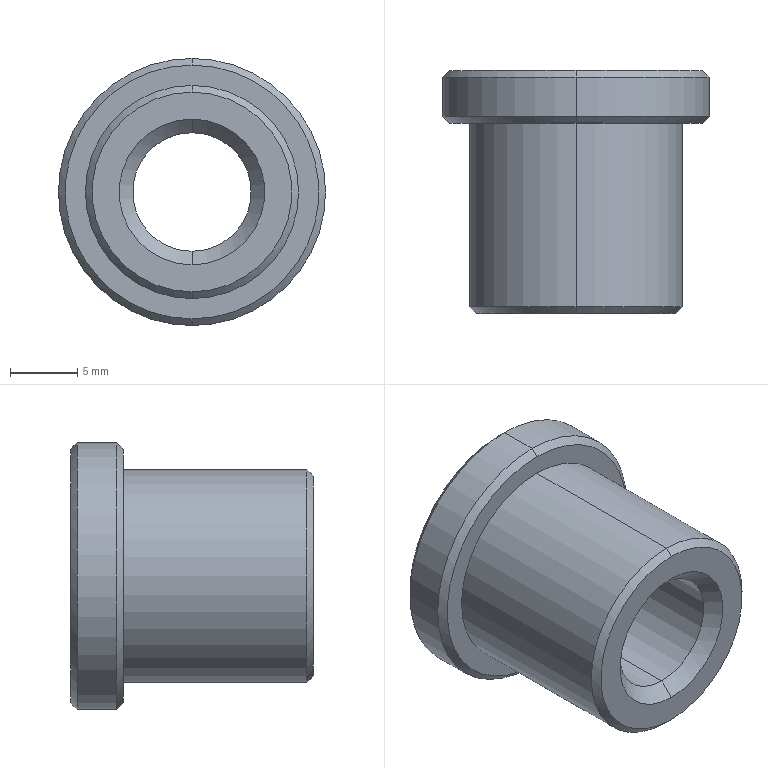Part | STEP file | BPSP-03-039Lift Joint | 1 solid | 19 faces | box 19.8 x 18 x 19.8 mm | volume 2819 mm3 | cone 10 | cylinder 6 | plane 3 | commonest cylinder face diameters 8.8 x2 15.8 x2 19.8 x2
STEP:
#1=CARTESIAN_POINT('',(0.,0.,0.));
#2=DIRECTION('',(0.,0.,1.));
#3=DIRECTION('',(1.,0.,0.));
#4=AXIS2_PLACEMENT_3D('',#1,#2,#3);
#5=CARTESIAN_POINT('',(0.,0.,-7.4));
#6=VERTEX_POINT('',#5);
#7=CARTESIAN_POINT('',(0.,0.,7.4));
#8=VERTEX_POINT('',#7);
#9=CARTESIAN_POINT('',(0.,0.,0.));
#10=DIRECTION('',(0.,-1.,0.));
#11=DIRECTION('',(0.,0.,-1.));
#12=AXIS2_PLACEMENT_3D('',#9,#10,#11);
#13=CIRCLE('',#12,7.4);
#14=CARTESIAN_POINT('',(0.,0.5,0.));
#15=DIRECTION('',(0.,1.,0.));
#16=DIRECTION('',(0.,0.,1.));
#17=AXIS2_PLACEMENT_3D('',#14,#15,#16);
#18=CONICAL_SURFACE('',#17,7.9,0.7854);
#19=CARTESIAN_POINT('',(3.142,-0.5));
#20=DIRECTION('',(-1.,0.));
#21=VECTOR('',#20,1.);
#22=LINE('',#19,#21);
#23=(GEOMETRIC_REPRESENTATION_CONTEXT(2)PARAMETRIC_REPRESENTATION_CONTEXT()REPRESENTATION_CONTEXT('',''));
#24=DEFINITIONAL_REPRESENTATION('',(#22),#23);
#25=PCURVE('',#18,#24);
#26=CARTESIAN_POINT('',(-4.,0.,0.));
#27=DIRECTION('',(0.,-1.,0.));
#28=DIRECTION('',(0.,0.,-1.));
#29=AXIS2_PLACEMENT_3D('',#26,#27,#28);
#30=PLANE('',#29);
#31=CARTESIAN_POINT('',(0.,4.));
#32=DIRECTION('',(1.,0.));
#33=AXIS2_PLACEMENT_2D('',#31,#32);
#34=CIRCLE('',#33,7.4);
#35=(GEOMETRIC_REPRESENTATION_CONTEXT(2)PARAMETRIC_REPRESENTATION_CONTEXT()REPRESENTATION_CONTEXT('',''));
#36=DEFINITIONAL_REPRESENTATION('',(#34),#35);
#37=PCURVE('',#30,#36);
#38=SURFACE_CURVE('',#13,(#25,#37),.PCURVE_S1.);
#39=EDGE_CURVE('',#6,#8,#38,.T.);
#40=ORIENTED_EDGE('',*,*,#39,.F.);
#41=CARTESIAN_POINT('',(0.,0.5,-7.9));
#42=VERTEX_POINT('',#41);
#43=CARTESIAN_POINT('',(0.,0.5,-7.9));
#44=DIRECTION('',(0.,0.7071,-0.7071));
#45=VECTOR('',#44,1.);
#46=LINE('',#43,#45);
#47=CARTESIAN_POINT('',(3.142,0.));
#48=DIRECTION('',(0.,1.));
#49=VECTOR('',#48,1.);
#50=LINE('',#47,#49);
#51=(GEOMETRIC_REPRESENTATION_CONTEXT(2)PARAMETRIC_REPRESENTATION_CONTEXT()REPRESENTATION_CONTEXT('',''));
#52=DEFINITIONAL_REPRESENTATION('',(#50),#51);
#53=PCURVE('',#18,#52);
#54=CARTESIAN_POINT('',(0.,0.5,0.));
#55=DIRECTION('',(0.,1.,0.));
#56=DIRECTION('',(0.,0.,1.));
#57=AXIS2_PLACEMENT_3D('',#54,#55,#56);
#58=CONICAL_SURFACE('',#57,7.9,0.7854);
#59=CARTESIAN_POINT('',(3.142,0.));
#60=DIRECTION('',(0.,1.));
#61=VECTOR('',#60,1.);
#62=LINE('',#59,#61);
#63=(GEOMETRIC_REPRESENTATION_CONTEXT(2)PARAMETRIC_REPRESENTATION_CONTEXT()REPRESENTATION_CONTEXT('',''));
#64=DEFINITIONAL_REPRESENTATION('',(#62),#63);
#65=PCURVE('',#58,#64);
#66=SURFACE_CURVE('',#46,(#53,#65),.PCURVE_S1.);
#67=EDGE_CURVE('',#6,#42,#66,.T.);
#68=ORIENTED_EDGE('',*,*,#67,.T.);
#69=CARTESIAN_POINT('',(0.,0.5,7.9));
#70=VERTEX_POINT('',#69);
#71=CARTESIAN_POINT('',(0.,0.5,0.));
#72=DIRECTION('',(0.,1.,0.));
#73=DIRECTION('',(0.,0.,-1.));
#74=AXIS2_PLACEMENT_3D('',#71,#72,#73);
#75=CIRCLE('',#74,7.9);
#76=CARTESIAN_POINT('',(-3.142,0.));
#77=DIRECTION('',(1.,0.));
#78=VECTOR('',#77,1.);
#79=LINE('',#76,#78);
#80=(GEOMETRIC_REPRESENTATION_CONTEXT(2)PARAMETRIC_REPRESENTATION_CONTEXT()REPRESENTATION_CONTEXT('',''));
#81=DEFINITIONAL_REPRESENTATION('',(#79),#80);
#82=PCURVE('',#18,#81);
#83=CARTESIAN_POINT('',(0.,-2.167,0.));
#84=DIRECTION('',(0.,1.,0.));
#85=DIRECTION('',(0.,0.,1.));
#86=AXIS2_PLACEMENT_3D('',#83,#84,#85);
#87=CYLINDRICAL_SURFACE('',#86,7.9);
#88=CARTESIAN_POINT('',(-3.142,2.667));
#89=DIRECTION('',(1.,0.));
#90=VECTOR('',#89,1.);
#91=LINE('',#88,#90);
#92=(GEOMETRIC_REPRESENTATION_CONTEXT(2)PARAMETRIC_REPRESENTATION_CONTEXT()REPRESENTATION_CONTEXT('',''));
#93=DEFINITIONAL_REPRESENTATION('',(#91),#92);
#94=PCURVE('',#87,#93);
#95=SURFACE_CURVE('',#75,(#82,#94),.PCURVE_S1.);
#96=EDGE_CURVE('',#70,#42,#95,.T.);
#97=ORIENTED_EDGE('',*,*,#96,.F.);
#98=CARTESIAN_POINT('',(0.,0.5,7.9));
#99=DIRECTION('',(0.,0.7071,0.7071));
#100=VECTOR('',#99,1.);
#101=LINE('',#98,#100);
#102=CARTESIAN_POINT('',(0.,0.));
#103=DIRECTION('',(0.,1.));
#104=VECTOR('',#103,1.);
#105=LINE('',#102,#104);
#106=(GEOMETRIC_REPRESENTATION_CONTEXT(2)PARAMETRIC_REPRESENTATION_CONTEXT()REPRESENTATION_CONTEXT('',''));
#107=DEFINITIONAL_REPRESENTATION('',(#105),#106);
#108=PCURVE('',#18,#107);
#109=CARTESIAN_POINT('',(6.283,0.));
#110=DIRECTION('',(0.,1.));
#111=VECTOR('',#110,1.);
#112=LINE('',#109,#111);
#113=(GEOMETRIC_REPRESENTATION_CONTEXT(2)PARAMETRIC_REPRESENTATION_CONTEXT()REPRESENTATION_CONTEXT('',''));
#114=DEFINITIONAL_REPRESENTATION('',(#112),#113);
#115=PCURVE('',#58,#114);
#116=SURFACE_CURVE('',#101,(#108,#115),.PCURVE_S1.);
#117=EDGE_CURVE('',#8,#70,#116,.T.);
#118=ORIENTED_EDGE('',*,*,#117,.F.);
#119=EDGE_LOOP('',(#40,#68,#97,#118));
#120=FACE_BOUND('',#119,.T.);
#121=ADVANCED_FACE('',(#120),#18,.T.);
#122=CARTESIAN_POINT('',(0.,14.1,-9.4));
#123=VERTEX_POINT('',#122);
#124=CARTESIAN_POINT('',(0.,14.1,9.4));
#125=VERTEX_POINT('',#124);
#126=CARTESIAN_POINT('',(0.,14.1,0.));
#127=DIRECTION('',(0.,-1.,0.));
#128=DIRECTION('',(0.,0.,-1.));
#129=AXIS2_PLACEMENT_3D('',#126,#127,#128);
#130=CIRCLE('',#129,9.4);
#131=CARTESIAN_POINT('',(0.,14.6,0.));
#132=DIRECTION('',(0.,1.,0.));
#133=DIRECTION('',(0.,0.,1.));
#134=AXIS2_PLACEMENT_3D('',#131,#132,#133);
#135=CONICAL_SURFACE('',#134,9.9,0.7854);
#136=CARTESIAN_POINT('',(3.142,-0.5));
#137=DIRECTION('',(-1.,0.));
#138=VECTOR('',#137,1.);
#139=LINE('',#136,#138);
#140=(GEOMETRIC_REPRESENTATION_CONTEXT(2)PARAMETRIC_REPRESENTATION_CONTEXT()REPRESENTATION_CONTEXT('',''));
#141=DEFINITIONAL_REPRESENTATION('',(#139),#140);
#142=PCURVE('',#135,#141);
#143=CARTESIAN_POINT('',(-7.9,14.1,0.));
#144=DIRECTION('',(0.,-1.,0.));
#145=DIRECTION('',(0.,0.,-1.));
#146=AXIS2_PLACEMENT_3D('',#143,#144,#145);
#147=PLANE('',#146);
#148=CARTESIAN_POINT('',(0.,7.9));
#149=DIRECTION('',(1.,0.));
#150=AXIS2_PLACEMENT_2D('',#148,#149);
#151=CIRCLE('',#150,9.4);
#152=(GEOMETRIC_REPRESENTATION_CONTEXT(2)PARAMETRIC_REPRESENTATION_CONTEXT()REPRESENTATION_CONTEXT('',''));
#153=DEFINITIONAL_REPRESENTATION('',(#151),#152);
#154=PCURVE('',#147,#153);
#155=SURFACE_CURVE('',#130,(#142,#154),.PCURVE_S1.);
#156=EDGE_CURVE('',#123,#125,#155,.T.);
#157=ORIENTED_EDGE('',*,*,#156,.F.);
#158=CARTESIAN_POINT('',(0.,14.6,-9.9));
#159=VERTEX_POINT('',#158);
#160=CARTESIAN_POINT('',(0.,14.6,-9.9));
#161=DIRECTION('',(0.,0.7071,-0.7071));
#162=VECTOR('',#161,1.);
#163=LINE('',#160,#162);
#164=CARTESIAN_POINT('',(3.142,0.));
#165=DIRECTION('',(0.,1.));
#166=VECTOR('',#165,1.);
#167=LINE('',#164,#166);
#168=(GEOMETRIC_REPRESENTATION_CONTEXT(2)PARAMETRIC_REPRESENTATION_CONTEXT()REPRESENTATION_CONTEXT('',''));
#169=DEFINITIONAL_REPRESENTATION('',(#167),#168);
#170=PCURVE('',#135,#169);
#171=CARTESIAN_POINT('',(0.,14.6,0.));
#172=DIRECTION('',(0.,1.,0.));
#173=DIRECTION('',(0.,0.,1.));
#174=AXIS2_PLACEMENT_3D('',#171,#172,#173);
#175=CONICAL_SURFACE('',#174,9.9,0.7854);
#176=CARTESIAN_POINT('',(3.142,0.));
#177=DIRECTION('',(0.,1.));
#178=VECTOR('',#177,1.);
#179=LINE('',#176,#178);
#180=(GEOMETRIC_REPRESENTATION_CONTEXT(2)PARAMETRIC_REPRESENTATION_CONTEXT()REPRESENTATION_CONTEXT('',''));
#181=DEFINITIONAL_REPRESENTATION('',(#179),#180);
#182=PCURVE('',#175,#181);
#183=SURFACE_CURVE('',#163,(#170,#182),.PCURVE_S1.);
#184=EDGE_CURVE('',#123,#159,#183,.T.);
#185=ORIENTED_EDGE('',*,*,#184,.T.);
#186=CARTESIAN_POINT('',(0.,14.6,9.9));
#187=VERTEX_POINT('',#186);
#188=CARTESIAN_POINT('',(0.,14.6,0.));
#189=DIRECTION('',(0.,1.,0.));
#190=DIRECTION('',(0.,0.,-1.));
#191=AXIS2_PLACEMENT_3D('',#188,#189,#190);
#192=CIRCLE('',#191,9.9);
#193=CARTESIAN_POINT('',(-3.142,0.));
#194=DIRECTION('',(1.,0.));
#195=VECTOR('',#194,1.);
#196=LINE('',#193,#195);
#197=(GEOMETRIC_REPRESENTATION_CONTEXT(2)PARAMETRIC_REPRESENTATION_CONTEXT()REPRESENTATION_CONTEXT('',''));
#198=DEFINITIONAL_REPRESENTATION('',(#196),#197);
#199=PCURVE('',#135,#198);
#200=CARTESIAN_POINT('',(0.,-2.167,0.));
#201=DIRECTION('',(0.,1.,0.));
#202=DIRECTION('',(0.,0.,1.));
#203=AXIS2_PLACEMENT_3D('',#200,#201,#202);
#204=CYLINDRICAL_SURFACE('',#203,9.9);
#205=CARTESIAN_POINT('',(-3.142,16.767));
#206=DIRECTION('',(1.,0.));
#207=VECTOR('',#206,1.);
#208=LINE('',#205,#207);
#209=(GEOMETRIC_REPRESENTATION_CONTEXT(2)PARAMETRIC_REPRESENTATION_CONTEXT()REPRESENTATION_CONTEXT('',''));
#210=DEFINITIONAL_REPRESENTATION('',(#208),#209);
#211=PCURVE('',#204,#210);
#212=SURFACE_CURVE('',#192,(#199,#211),.PCURVE_S1.);
#213=EDGE_CURVE('',#187,#159,#212,.T.);
#214=ORIENTED_EDGE('',*,*,#213,.F.);
#215=CARTESIAN_POINT('',(0.,14.6,9.9));
#216=DIRECTION('',(0.,0.7071,0.7071));
#217=VECTOR('',#216,1.);
#218=LINE('',#215,#217);
#219=CARTESIAN_POINT('',(0.,0.));
#220=DIRECTION('',(0.,1.));
#221=VECTOR('',#220,1.);
#222=LINE('',#219,#221);
#223=(GEOMETRIC_REPRESENTATION_CONTEXT(2)PARAMETRIC_REPRESENTATION_CONTEXT()REPRESENTATION_CONTEXT('',''));
#224=DEFINITIONAL_REPRESENTATION('',(#222),#223);
#225=PCURVE('',#135,#224);
#226=CARTESIAN_POINT('',(6.283,0.));
#227=DIRECTION('',(0.,1.));
#228=VECTOR('',#227,1.);
#229=LINE('',#226,#228);
#230=(GEOMETRIC_REPRESENTATION_CONTEXT(2)PARAMETRIC_REPRESENTATION_CONTEXT()REPRESENTATION_CONTEXT('',''));
#231=DEFINITIONAL_REPRESENTATION('',(#229),#230);
#232=PCURVE('',#175,#231);
#233=SURFACE_CURVE('',#218,(#225,#232),.PCURVE_S1.);
#234=EDGE_CURVE('',#125,#187,#233,.T.);
#235=ORIENTED_EDGE('',*,*,#234,.F.);
#236=EDGE_LOOP('',(#157,#185,#214,#235));
#237=FACE_BOUND('',#236,.T.);
#238=ADVANCED_FACE('',(#237),#135,.T.);
#239=CARTESIAN_POINT('',(0.,18.,9.4));
#240=VERTEX_POINT('',#239);
#241=CARTESIAN_POINT('',(0.,18.,-9.4));
#242=VERTEX_POINT('',#241);
#243=CARTESIAN_POINT('',(0.,18.,0.));
#244=DIRECTION('',(0.,1.,0.));
#245=DIRECTION('',(0.,0.,1.));
#246=AXIS2_PLACEMENT_3D('',#243,#244,#245);
#247=CIRCLE('',#246,9.4);
#248=CARTESIAN_POINT('',(0.,18.,0.));
#249=DIRECTION('',(0.,-1.,0.));
#250=DIRECTION('',(0.,0.,-1.));
#251=AXIS2_PLACEMENT_3D('',#248,#249,#250);
#252=CONICAL_SURFACE('',#251,9.4,0.7854);
#253=CARTESIAN_POINT('',(3.142,0.));
#254=DIRECTION('',(-1.,0.));
#255=VECTOR('',#254,1.);
#256=LINE('',#253,#255);
#257=(GEOMETRIC_REPRESENTATION_CONTEXT(2)PARAMETRIC_REPRESENTATION_CONTEXT()REPRESENTATION_CONTEXT('',''));
#258=DEFINITIONAL_REPRESENTATION('',(#256),#257);
#259=PCURVE('',#252,#258);
#260=CARTESIAN_POINT('',(-9.9,18.,0.));
#261=DIRECTION('',(0.,1.,0.));
#262=DIRECTION('',(0.,0.,1.));
#263=AXIS2_PLACEMENT_3D('',#260,#261,#262);
#264=PLANE('',#263);
#265=CARTESIAN_POINT('',(0.,9.9));
#266=DIRECTION('',(1.,0.));
#267=AXIS2_PLACEMENT_2D('',#265,#266);
#268=CIRCLE('',#267,9.4);
#269=(GEOMETRIC_REPRESENTATION_CONTEXT(2)PARAMETRIC_REPRESENTATION_CONTEXT()REPRESENTATION_CONTEXT('',''));
#270=DEFINITIONAL_REPRESENTATION('',(#268),#269);
#271=PCURVE('',#264,#270);
#272=SURFACE_CURVE('',#247,(#259,#271),.PCURVE_S1.);
#273=EDGE_CURVE('',#240,#242,#272,.T.);
#274=ORIENTED_EDGE('',*,*,#273,.F.);
#275=CARTESIAN_POINT('',(0.,17.5,9.9));
#276=VERTEX_POINT('',#275);
#277=CARTESIAN_POINT('',(0.,18.,9.4));
#278=DIRECTION('',(0.,-0.7071,0.7071));
#279=VECTOR('',#278,1.);
#280=LINE('',#277,#279);
#281=CARTESIAN_POINT('',(3.142,0.));
#282=DIRECTION('',(0.,1.));
#283=VECTOR('',#282,1.);
#284=LINE('',#281,#283);
#285=(GEOMETRIC_REPRESENTATION_CONTEXT(2)PARAMETRIC_REPRESENTATION_CONTEXT()REPRESENTATION_CONTEXT('',''));
#286=DEFINITIONAL_REPRESENTATION('',(#284),#285);
#287=PCURVE('',#252,#286);
#288=CARTESIAN_POINT('',(0.,18.,0.));
#289=DIRECTION('',(0.,-1.,0.));
#290=DIRECTION('',(0.,0.,-1.));
#291=AXIS2_PLACEMENT_3D('',#288,#289,#290);
#292=CONICAL_SURFACE('',#291,9.4,0.7854);
#293=CARTESIAN_POINT('',(3.142,0.));
#294=DIRECTION('',(0.,1.));
#295=VECTOR('',#294,1.);
#296=LINE('',#293,#295);
#297=(GEOMETRIC_REPRESENTATION_CONTEXT(2)PARAMETRIC_REPRESENTATION_CONTEXT()REPRESENTATION_CONTEXT('',''));
#298=DEFINITIONAL_REPRESENTATION('',(#296),#297);
#299=PCURVE('',#292,#298);
#300=SURFACE_CURVE('',#280,(#287,#299),.PCURVE_S1.);
#301=EDGE_CURVE('',#240,#276,#300,.T.);
#302=ORIENTED_EDGE('',*,*,#301,.T.);
#303=CARTESIAN_POINT('',(0.,17.5,-9.9));
#304=VERTEX_POINT('',#303);
#305=CARTESIAN_POINT('',(0.,17.5,0.));
#306=DIRECTION('',(0.,-1.,0.));
#307=DIRECTION('',(0.,0.,1.));
#308=AXIS2_PLACEMENT_3D('',#305,#306,#307);
#309=CIRCLE('',#308,9.9);
#310=CARTESIAN_POINT('',(-3.142,0.5));
#311=DIRECTION('',(1.,0.));
#312=VECTOR('',#311,1.);
#313=LINE('',#310,#312);
#314=(GEOMETRIC_REPRESENTATION_CONTEXT(2)PARAMETRIC_REPRESENTATION_CONTEXT()REPRESENTATION_CONTEXT('',''));
#315=DEFINITIONAL_REPRESENTATION('',(#313),#314);
#316=PCURVE('',#252,#315);
#317=CARTESIAN_POINT('',(6.283,19.667));
#318=DIRECTION('',(-1.,0.));
#319=VECTOR('',#318,1.);
#320=LINE('',#317,#319);
#321=(GEOMETRIC_REPRESENTATION_CONTEXT(2)PARAMETRIC_REPRESENTATION_CONTEXT()REPRESENTATION_CONTEXT('',''));
#322=DEFINITIONAL_REPRESENTATION('',(#320),#321);
#323=PCURVE('',#204,#322);
#324=SURFACE_CURVE('',#309,(#316,#323),.PCURVE_S1.);
#325=EDGE_CURVE('',#304,#276,#324,.T.);
#326=ORIENTED_EDGE('',*,*,#325,.F.);
#327=CARTESIAN_POINT('',(0.,18.,-9.4));
#328=DIRECTION('',(0.,-0.7071,-0.7071));
#329=VECTOR('',#328,1.);
#330=LINE('',#327,#329);
#331=CARTESIAN_POINT('',(0.,0.));
#332=DIRECTION('',(0.,1.));
#333=VECTOR('',#332,1.);
#334=LINE('',#331,#333);
#335=(GEOMETRIC_REPRESENTATION_CONTEXT(2)PARAMETRIC_REPRESENTATION_CONTEXT()REPRESENTATION_CONTEXT('',''));
#336=DEFINITIONAL_REPRESENTATION('',(#334),#335);
#337=PCURVE('',#252,#336);
#338=CARTESIAN_POINT('',(6.283,0.));
#339=DIRECTION('',(0.,1.));
#340=VECTOR('',#339,1.);
#341=LINE('',#338,#340);
#342=(GEOMETRIC_REPRESENTATION_CONTEXT(2)PARAMETRIC_REPRESENTATION_CONTEXT()REPRESENTATION_CONTEXT('',''));
#343=DEFINITIONAL_REPRESENTATION('',(#341),#342);
#344=PCURVE('',#292,#343);
#345=SURFACE_CURVE('',#330,(#337,#344),.PCURVE_S1.);
#346=EDGE_CURVE('',#242,#304,#345,.T.);
#347=ORIENTED_EDGE('',*,*,#346,.F.);
#348=EDGE_LOOP('',(#274,#302,#326,#347));
#349=FACE_BOUND('',#348,.T.);
#350=ADVANCED_FACE('',(#349),#252,.T.);
#351=CARTESIAN_POINT('',(0.,17.,4.4));
#352=VERTEX_POINT('',#351);
#353=CARTESIAN_POINT('',(0.,18.,5.4));
#354=VERTEX_POINT('',#353);
#355=CARTESIAN_POINT('',(0.,18.,5.4));
#356=DIRECTION('',(0.,0.7071,0.7071));
#357=VECTOR('',#356,1.);
#358=LINE('',#355,#357);
#359=CARTESIAN_POINT('',(0.,18.,0.));
#360=DIRECTION('',(0.,1.,0.));
#361=DIRECTION('',(0.,0.,1.));
#362=AXIS2_PLACEMENT_3D('',#359,#360,#361);
#363=CONICAL_SURFACE('',#362,5.4,0.7854);
#364=CARTESIAN_POINT('',(6.283,0.));
#365=DIRECTION('',(0.,1.));
#366=VECTOR('',#365,1.);
#367=LINE('',#364,#366);
#368=(GEOMETRIC_REPRESENTATION_CONTEXT(2)PARAMETRIC_REPRESENTATION_CONTEXT()REPRESENTATION_CONTEXT('',''));
#369=DEFINITIONAL_REPRESENTATION('',(#367),#368);
#370=PCURVE('',#363,#369);
#371=CARTESIAN_POINT('',(0.,18.,0.));
#372=DIRECTION('',(0.,1.,0.));
#373=DIRECTION('',(0.,0.,1.));
#374=AXIS2_PLACEMENT_3D('',#371,#372,#373);
#375=CONICAL_SURFACE('',#374,5.4,0.7854);
#376=CARTESIAN_POINT('',(0.,0.));
#377=DIRECTION('',(0.,1.));
#378=VECTOR('',#377,1.);
#379=LINE('',#376,#378);
#380=(GEOMETRIC_REPRESENTATION_CONTEXT(2)PARAMETRIC_REPRESENTATION_CONTEXT()REPRESENTATION_CONTEXT('',''));
#381=DEFINITIONAL_REPRESENTATION('',(#379),#380);
#382=PCURVE('',#375,#381);
#383=SURFACE_CURVE('',#358,(#370,#382),.PCURVE_S1.);
#384=EDGE_CURVE('',#352,#354,#383,.T.);
#385=ORIENTED_EDGE('',*,*,#384,.T.);
#386=CARTESIAN_POINT('',(0.,18.,-5.4));
#387=VERTEX_POINT('',#386);
#388=CARTESIAN_POINT('',(0.,18.,0.));
#389=DIRECTION('',(0.,-1.,0.));
#390=DIRECTION('',(0.,0.,1.));
#391=AXIS2_PLACEMENT_3D('',#388,#389,#390);
#392=CIRCLE('',#391,5.4);
#393=CARTESIAN_POINT('',(6.283,0.));
#394=DIRECTION('',(-1.,0.));
#395=VECTOR('',#394,1.);
#396=LINE('',#393,#395);
#397=(GEOMETRIC_REPRESENTATION_CONTEXT(2)PARAMETRIC_REPRESENTATION_CONTEXT()REPRESENTATION_CONTEXT('',''));
#398=DEFINITIONAL_REPRESENTATION('',(#396),#397);
#399=PCURVE('',#363,#398);
#400=CARTESIAN_POINT('',(5.4,9.9));
#401=CARTESIAN_POINT('',(5.4,0.5469));
#402=CARTESIAN_POINT('',(-2.7,5.223));
#403=CARTESIAN_POINT('',(-10.8,9.9));
#404=CARTESIAN_POINT('',(-2.7,14.577));
#405=CARTESIAN_POINT('',(5.4,19.253));
#406=CARTESIAN_POINT('',(5.4,9.9));
#407=(BOUNDED_CURVE()B_SPLINE_CURVE(2,(#400,#401,#402,#403,#404,#405,#406),.UNSPECIFIED.,.T.,.F.)B_SPLINE_CURVE_WITH_KNOTS((1,2,2,2,2,1),(-2.094,0.,2.094,4.189,6.283,8.378),.UNSPECIFIED.)CURVE()GEOMETRIC_REPRESENTATION_ITEM()RATIONAL_B_SPLINE_CURVE((1.,0.5,1.,0.5,1.,0.5,1.))REPRESENTATION_ITEM(''));
#408=(GEOMETRIC_REPRESENTATION_CONTEXT(2)PARAMETRIC_REPRESENTATION_CONTEXT()REPRESENTATION_CONTEXT('',''));
#409=DEFINITIONAL_REPRESENTATION('',(#407),#408);
#410=PCURVE('',#264,#409);
#411=SURFACE_CURVE('',#392,(#399,#410),.PCURVE_S1.);
#412=EDGE_CURVE('',#354,#387,#411,.T.);
#413=ORIENTED_EDGE('',*,*,#412,.T.);
#414=CARTESIAN_POINT('',(0.,17.,-4.4));
#415=VERTEX_POINT('',#414);
#416=CARTESIAN_POINT('',(0.,18.,-5.4));
#417=DIRECTION('',(0.,0.7071,-0.7071));
#418=VECTOR('',#417,1.);
#419=LINE('',#416,#418);
#420=CARTESIAN_POINT('',(3.142,0.));
#421=DIRECTION('',(0.,1.));
#422=VECTOR('',#421,1.);
#423=LINE('',#420,#422);
#424=(GEOMETRIC_REPRESENTATION_CONTEXT(2)PARAMETRIC_REPRESENTATION_CONTEXT()REPRESENTATION_CONTEXT('',''));
#425=DEFINITIONAL_REPRESENTATION('',(#423),#424);
#426=PCURVE('',#363,#425);
#427=CARTESIAN_POINT('',(3.142,0.));
#428=DIRECTION('',(0.,1.));
#429=VECTOR('',#428,1.);
#430=LINE('',#427,#429);
#431=(GEOMETRIC_REPRESENTATION_CONTEXT(2)PARAMETRIC_REPRESENTATION_CONTEXT()REPRESENTATION_CONTEXT('',''));
#432=DEFINITIONAL_REPRESENTATION('',(#430),#431);
#433=PCURVE('',#375,#432);
#434=SURFACE_CURVE('',#419,(#426,#433),.PCURVE_S1.);
#435=EDGE_CURVE('',#415,#387,#434,.T.);
#436=ORIENTED_EDGE('',*,*,#435,.F.);
#437=CARTESIAN_POINT('',(0.,17.,0.));
#438=DIRECTION('',(0.,1.,0.));
#439=DIRECTION('',(0.,0.,1.));
#440=AXIS2_PLACEMENT_3D('',#437,#438,#439);
#441=CIRCLE('',#440,4.4);
#442=CARTESIAN_POINT('',(0.,-1.));
#443=DIRECTION('',(1.,0.));
#444=VECTOR('',#443,1.);
#445=LINE('',#442,#444);
#446=(GEOMETRIC_REPRESENTATION_CONTEXT(2)PARAMETRIC_REPRESENTATION_CONTEXT()REPRESENTATION_CONTEXT('',''));
#447=DEFINITIONAL_REPRESENTATION('',(#445),#446);
#448=PCURVE('',#363,#447);
#449=CARTESIAN_POINT('',(0.,0.,0.));
#450=DIRECTION('',(0.,-1.,0.));
#451=DIRECTION('',(0.,0.,-1.));
#452=AXIS2_PLACEMENT_3D('',#449,#450,#451);
#453=CYLINDRICAL_SURFACE('',#452,4.4);
#454=CARTESIAN_POINT('',(9.425,-17.));
#455=DIRECTION('',(-1.,0.));
#456=VECTOR('',#455,1.);
#457=LINE('',#454,#456);
#458=(GEOMETRIC_REPRESENTATION_CONTEXT(2)PARAMETRIC_REPRESENTATION_CONTEXT()REPRESENTATION_CONTEXT('',''));
#459=DEFINITIONAL_REPRESENTATION('',(#457),#458);
#460=PCURVE('',#453,#459);
#461=SURFACE_CURVE('',#441,(#448,#460),.PCURVE_S1.);
#462=EDGE_CURVE('',#415,#352,#461,.T.);
#463=ORIENTED_EDGE('',*,*,#462,.T.);
#464=EDGE_LOOP('',(#385,#413,#436,#463));
#465=FACE_BOUND('',#464,.F.);
#466=ADVANCED_FACE('',(#465),#363,.F.);
#467=CARTESIAN_POINT('',(0.,1.,-4.4));
#468=VERTEX_POINT('',#467);
#469=CARTESIAN_POINT('',(0.,0.,-5.4));
#470=VERTEX_POINT('',#469);
#471=CARTESIAN_POINT('',(0.,1.,-4.4));
#472=DIRECTION('',(0.,-0.7071,-0.7071));
#473=VECTOR('',#472,1.);
#474=LINE('',#471,#473);
#475=CARTESIAN_POINT('',(0.,1.,0.));
#476=DIRECTION('',(0.,-1.,0.));
#477=DIRECTION('',(0.,0.,-1.));
#478=AXIS2_PLACEMENT_3D('',#475,#476,#477);
#479=CONICAL_SURFACE('',#478,4.4,0.7854);
#480=CARTESIAN_POINT('',(6.283,0.));
#481=DIRECTION('',(0.,1.));
#482=VECTOR('',#481,1.);
#483=LINE('',#480,#482);
#484=(GEOMETRIC_REPRESENTATION_CONTEXT(2)PARAMETRIC_REPRESENTATION_CONTEXT()REPRESENTATION_CONTEXT('',''));
#485=DEFINITIONAL_REPRESENTATION('',(#483),#484);
#486=PCURVE('',#479,#485);
#487=CARTESIAN_POINT('',(0.,1.,0.));
#488=DIRECTION('',(0.,-1.,0.));
#489=DIRECTION('',(0.,0.,-1.));
#490=AXIS2_PLACEMENT_3D('',#487,#488,#489);
#491=CONICAL_SURFACE('',#490,4.4,0.7854);
#492=CARTESIAN_POINT('',(0.,0.));
#493=DIRECTION('',(0.,1.));
#494=VECTOR('',#493,1.);
#495=LINE('',#492,#494);
#496=(GEOMETRIC_REPRESENTATION_CONTEXT(2)PARAMETRIC_REPRESENTATION_CONTEXT()REPRESENTATION_CONTEXT('',''));
#497=DEFINITIONAL_REPRESENTATION('',(#495),#496);
#498=PCURVE('',#491,#497);
#499=SURFACE_CURVE('',#474,(#486,#498),.PCURVE_S1.);
#500=EDGE_CURVE('',#468,#470,#499,.T.);
#501=ORIENTED_EDGE('',*,*,#500,.T.);
#502=CARTESIAN_POINT('',(0.,0.,5.4));
#503=VERTEX_POINT('',#502);
#504=CARTESIAN_POINT('',(0.,0.,0.));
#505=DIRECTION('',(0.,1.,0.));
#506=DIRECTION('',(0.,0.,-1.));
#507=AXIS2_PLACEMENT_3D('',#504,#505,#506);
#508=CIRCLE('',#507,5.4);
#509=CARTESIAN_POINT('',(6.283,1.));
#510=DIRECTION('',(-1.,0.));
#511=VECTOR('',#510,1.);
#512=LINE('',#509,#511);
#513=(GEOMETRIC_REPRESENTATION_CONTEXT(2)PARAMETRIC_REPRESENTATION_CONTEXT()REPRESENTATION_CONTEXT('',''));
#514=DEFINITIONAL_REPRESENTATION('',(#512),#513);
#515=PCURVE('',#479,#514);
#516=CARTESIAN_POINT('',(5.4,4.));
#517=CARTESIAN_POINT('',(5.4,-5.353));
#518=CARTESIAN_POINT('',(-2.7,-0.6765));
#519=CARTESIAN_POINT('',(-10.8,4.));
#520=CARTESIAN_POINT('',(-2.7,8.677));
#521=CARTESIAN_POINT('',(5.4,13.353));
#522=CARTESIAN_POINT('',(5.4,4.));
#523=(BOUNDED_CURVE()B_SPLINE_CURVE(2,(#516,#517,#518,#519,#520,#521,#522),.UNSPECIFIED.,.T.,.F.)B_SPLINE_CURVE_WITH_KNOTS((1,2,2,2,2,1),(-2.094,0.,2.094,4.189,6.283,8.378),.UNSPECIFIED.)CURVE()GEOMETRIC_REPRESENTATION_ITEM()RATIONAL_B_SPLINE_CURVE((1.,0.5,1.,0.5,1.,0.5,1.))REPRESENTATION_ITEM(''));
#524=(GEOMETRIC_REPRESENTATION_CONTEXT(2)PARAMETRIC_REPRESENTATION_CONTEXT()REPRESENTATION_CONTEXT('',''));
#525=DEFINITIONAL_REPRESENTATION('',(#523),#524);
#526=PCURVE('',#30,#525);
#527=SURFACE_CURVE('',#508,(#515,#526),.PCURVE_S1.);
#528=EDGE_CURVE('',#470,#503,#527,.T.);
#529=ORIENTED_EDGE('',*,*,#528,.T.);
#530=CARTESIAN_POINT('',(0.,1.,4.4));
#531=VERTEX_POINT('',#530);
#532=CARTESIAN_POINT('',(0.,1.,4.4));
#533=DIRECTION('',(0.,-0.7071,0.7071));
#534=VECTOR('',#533,1.);
#535=LINE('',#532,#534);
#536=CARTESIAN_POINT('',(3.142,0.));
#537=DIRECTION('',(0.,1.));
#538=VECTOR('',#537,1.);
#539=LINE('',#536,#538);
#540=(GEOMETRIC_REPRESENTATION_CONTEXT(2)PARAMETRIC_REPRESENTATION_CONTEXT()REPRESENTATION_CONTEXT('',''));
#541=DEFINITIONAL_REPRESENTATION('',(#539),#540);
#542=PCURVE('',#479,#541);
#543=CARTESIAN_POINT('',(3.142,0.));
#544=DIRECTION('',(0.,1.));
#545=VECTOR('',#544,1.);
#546=LINE('',#543,#545);
#547=(GEOMETRIC_REPRESENTATION_CONTEXT(2)PARAMETRIC_REPRESENTATION_CONTEXT()REPRESENTATION_CONTEXT('',''));
#548=DEFINITIONAL_REPRESENTATION('',(#546),#547);
#549=PCURVE('',#491,#548);
#550=SURFACE_CURVE('',#535,(#542,#549),.PCURVE_S1.);
#551=EDGE_CURVE('',#531,#503,#550,.T.);
#552=ORIENTED_EDGE('',*,*,#551,.F.);
#553=CARTESIAN_POINT('',(0.,1.,0.));
#554=DIRECTION('',(0.,-1.,0.));
#555=DIRECTION('',(0.,0.,-1.));
#556=AXIS2_PLACEMENT_3D('',#553,#554,#555);
#557=CIRCLE('',#556,4.4);
#558=CARTESIAN_POINT('',(0.,0.));
#559=DIRECTION('',(1.,0.));
#560=VECTOR('',#559,1.);
#561=LINE('',#558,#560);
#562=(GEOMETRIC_REPRESENTATION_CONTEXT(2)PARAMETRIC_REPRESENTATION_CONTEXT()REPRESENTATION_CONTEXT('',''));
#563=DEFINITIONAL_REPRESENTATION('',(#561),#562);
#564=PCURVE('',#479,#563);
#565=CARTESIAN_POINT('',(0.,-1.));
#566=DIRECTION('',(1.,0.));
#567=VECTOR('',#566,1.);
#568=LINE('',#565,#567);
#569=(GEOMETRIC_REPRESENTATION_CONTEXT(2)PARAMETRIC_REPRESENTATION_CONTEXT()REPRESENTATION_CONTEXT('',''));
#570=DEFINITIONAL_REPRESENTATION('',(#568),#569);
#571=PCURVE('',#453,#570);
#572=SURFACE_CURVE('',#557,(#564,#571),.PCURVE_S1.);
#573=EDGE_CURVE('',#531,#468,#572,.T.);
#574=ORIENTED_EDGE('',*,*,#573,.T.);
#575=EDGE_LOOP('',(#501,#529,#552,#574));
#576=FACE_BOUND('',#575,.F.);
#577=ADVANCED_FACE('',(#576),#479,.F.);
#578=CARTESIAN_POINT('',(0.,0.,-4.4));
#579=DIRECTION('',(0.,-1.,0.));
#580=VECTOR('',#579,1.);
#581=LINE('',#578,#580);
#582=CARTESIAN_POINT('',(6.283,0.));
#583=DIRECTION('',(0.,1.));
#584=VECTOR('',#583,1.);
#585=LINE('',#582,#584);
#586=(GEOMETRIC_REPRESENTATION_CONTEXT(2)PARAMETRIC_REPRESENTATION_CONTEXT()REPRESENTATION_CONTEXT('',''));
#587=DEFINITIONAL_REPRESENTATION('',(#585),#586);
#588=PCURVE('',#453,#587);
#589=CARTESIAN_POINT('',(0.,0.,0.));
#590=DIRECTION('',(0.,-1.,0.));
#591=DIRECTION('',(0.,0.,-1.));
#592=AXIS2_PLACEMENT_3D('',#589,#590,#591);
#593=CYLINDRICAL_SURFACE('',#592,4.4);
#594=CARTESIAN_POINT('',(0.,0.));
#595=DIRECTION('',(0.,1.));
#596=VECTOR('',#595,1.);
#597=LINE('',#594,#596);
#598=(GEOMETRIC_REPRESENTATION_CONTEXT(2)PARAMETRIC_REPRESENTATION_CONTEXT()REPRESENTATION_CONTEXT('',''));
#599=DEFINITIONAL_REPRESENTATION('',(#597),#598);
#600=PCURVE('',#593,#599);
#601=SURFACE_CURVE('',#581,(#588,#600),.PCURVE_S1.);
#602=EDGE_CURVE('',#415,#468,#601,.T.);
#603=ORIENTED_EDGE('',*,*,#602,.T.);
#604=ORIENTED_EDGE('',*,*,#573,.F.);
#605=CARTESIAN_POINT('',(0.,0.,4.4));
#606=DIRECTION('',(0.,-1.,0.));
#607=VECTOR('',#606,1.);
#608=LINE('',#605,#607);
#609=CARTESIAN_POINT('',(3.142,0.));
#610=DIRECTION('',(0.,1.));
#611=VECTOR('',#610,1.);
#612=LINE('',#609,#611);
#613=(GEOMETRIC_REPRESENTATION_CONTEXT(2)PARAMETRIC_REPRESENTATION_CONTEXT()REPRESENTATION_CONTEXT('',''));
#614=DEFINITIONAL_REPRESENTATION('',(#612),#613);
#615=PCURVE('',#453,#614);
#616=CARTESIAN_POINT('',(3.142,0.));
#617=DIRECTION('',(0.,1.));
#618=VECTOR('',#617,1.);
#619=LINE('',#616,#618);
#620=(GEOMETRIC_REPRESENTATION_CONTEXT(2)PARAMETRIC_REPRESENTATION_CONTEXT()REPRESENTATION_CONTEXT('',''));
#621=DEFINITIONAL_REPRESENTATION('',(#619),#620);
#622=PCURVE('',#593,#621);
#623=SURFACE_CURVE('',#608,(#615,#622),.PCURVE_S1.);
#624=EDGE_CURVE('',#352,#531,#623,.T.);
#625=ORIENTED_EDGE('',*,*,#624,.F.);
#626=ORIENTED_EDGE('',*,*,#462,.F.);
#627=EDGE_LOOP('',(#603,#604,#625,#626));
#628=FACE_BOUND('',#627,.F.);
#629=ADVANCED_FACE('',(#628),#453,.F.);
#630=ORIENTED_EDGE('',*,*,#213,.T.);
#631=CARTESIAN_POINT('',(0.,-2.167,-9.9));
#632=DIRECTION('',(0.,1.,0.));
#633=VECTOR('',#632,1.);
#634=LINE('',#631,#633);
#635=CARTESIAN_POINT('',(3.142,0.));
#636=DIRECTION('',(0.,1.));
#637=VECTOR('',#636,1.);
#638=LINE('',#635,#637);
#639=(GEOMETRIC_REPRESENTATION_CONTEXT(2)PARAMETRIC_REPRESENTATION_CONTEXT()REPRESENTATION_CONTEXT('',''));
#640=DEFINITIONAL_REPRESENTATION('',(#638),#639);
#641=PCURVE('',#204,#640);
#642=CARTESIAN_POINT('',(0.,-2.167,0.));
#643=DIRECTION('',(0.,1.,0.));
#644=DIRECTION('',(0.,0.,1.));
#645=AXIS2_PLACEMENT_3D('',#642,#643,#644);
#646=CYLINDRICAL_SURFACE('',#645,9.9);
#647=CARTESIAN_POINT('',(3.142,0.));
#648=DIRECTION('',(0.,1.));
#649=VECTOR('',#648,1.);
#650=LINE('',#647,#649);
#651=(GEOMETRIC_REPRESENTATION_CONTEXT(2)PARAMETRIC_REPRESENTATION_CONTEXT()REPRESENTATION_CONTEXT('',''));
#652=DEFINITIONAL_REPRESENTATION('',(#650),#651);
#653=PCURVE('',#646,#652);
#654=SURFACE_CURVE('',#634,(#641,#653),.PCURVE_S1.);
#655=EDGE_CURVE('',#159,#304,#654,.T.);
#656=ORIENTED_EDGE('',*,*,#655,.T.);
#657=ORIENTED_EDGE('',*,*,#325,.T.);
#658=CARTESIAN_POINT('',(0.,-2.167,9.9));
#659=DIRECTION('',(0.,1.,0.));
#660=VECTOR('',#659,1.);
#661=LINE('',#658,#660);
#662=CARTESIAN_POINT('',(0.,0.));
#663=DIRECTION('',(0.,1.));
#664=VECTOR('',#663,1.);
#665=LINE('',#662,#664);
#666=(GEOMETRIC_REPRESENTATION_CONTEXT(2)PARAMETRIC_REPRESENTATION_CONTEXT()REPRESENTATION_CONTEXT('',''));
#667=DEFINITIONAL_REPRESENTATION('',(#665),#666);
#668=PCURVE('',#204,#667);
#669=CARTESIAN_POINT('',(6.283,0.));
#670=DIRECTION('',(0.,1.));
#671=VECTOR('',#670,1.);
#672=LINE('',#669,#671);
#673=(GEOMETRIC_REPRESENTATION_CONTEXT(2)PARAMETRIC_REPRESENTATION_CONTEXT()REPRESENTATION_CONTEXT('',''));
#674=DEFINITIONAL_REPRESENTATION('',(#672),#673);
#675=PCURVE('',#646,#674);
#676=SURFACE_CURVE('',#661,(#668,#675),.PCURVE_S1.);
#677=EDGE_CURVE('',#187,#276,#676,.T.);
#678=ORIENTED_EDGE('',*,*,#677,.F.);
#679=EDGE_LOOP('',(#630,#656,#657,#678));
#680=FACE_BOUND('',#679,.T.);
#681=ADVANCED_FACE('',(#680),#204,.T.);
#682=ORIENTED_EDGE('',*,*,#96,.T.);
#683=CARTESIAN_POINT('',(0.,14.1,-7.9));
#684=VERTEX_POINT('',#683);
#685=CARTESIAN_POINT('',(0.,-2.167,-7.9));
#686=DIRECTION('',(0.,1.,0.));
#687=VECTOR('',#686,1.);
#688=LINE('',#685,#687);
#689=CARTESIAN_POINT('',(3.142,0.));
#690=DIRECTION('',(0.,1.));
#691=VECTOR('',#690,1.);
#692=LINE('',#689,#691);
#693=(GEOMETRIC_REPRESENTATION_CONTEXT(2)PARAMETRIC_REPRESENTATION_CONTEXT()REPRESENTATION_CONTEXT('',''));
#694=DEFINITIONAL_REPRESENTATION('',(#692),#693);
#695=PCURVE('',#87,#694);
#696=CARTESIAN_POINT('',(0.,-2.167,0.));
#697=DIRECTION('',(0.,1.,0.));
#698=DIRECTION('',(0.,0.,1.));
#699=AXIS2_PLACEMENT_3D('',#696,#697,#698);
#700=CYLINDRICAL_SURFACE('',#699,7.9);
#701=CARTESIAN_POINT('',(3.142,0.));
#702=DIRECTION('',(0.,1.));
#703=VECTOR('',#702,1.);
#704=LINE('',#701,#703);
#705=(GEOMETRIC_REPRESENTATION_CONTEXT(2)PARAMETRIC_REPRESENTATION_CONTEXT()REPRESENTATION_CONTEXT('',''));
#706=DEFINITIONAL_REPRESENTATION('',(#704),#705);
#707=PCURVE('',#700,#706);
#708=SURFACE_CURVE('',#688,(#695,#707),.PCURVE_S1.);
#709=EDGE_CURVE('',#42,#684,#708,.T.);
#710=ORIENTED_EDGE('',*,*,#709,.T.);
#711=CARTESIAN_POINT('',(0.,14.1,7.9));
#712=VERTEX_POINT('',#711);
#713=CARTESIAN_POINT('',(0.,14.1,0.));
#714=DIRECTION('',(0.,1.,0.));
#715=DIRECTION('',(0.,0.,1.));
#716=AXIS2_PLACEMENT_3D('',#713,#714,#715);
#717=CIRCLE('',#716,7.9);
#718=CARTESIAN_POINT('',(0.,16.267));
#719=DIRECTION('',(1.,0.));
#720=VECTOR('',#719,1.);
#721=LINE('',#718,#720);
#722=(GEOMETRIC_REPRESENTATION_CONTEXT(2)PARAMETRIC_REPRESENTATION_CONTEXT()REPRESENTATION_CONTEXT('',''));
#723=DEFINITIONAL_REPRESENTATION('',(#721),#722);
#724=PCURVE('',#87,#723);
#725=CARTESIAN_POINT('',(-7.9,7.9));
#726=CARTESIAN_POINT('',(-7.9,21.583));
#727=CARTESIAN_POINT('',(3.95,14.742));
#728=CARTESIAN_POINT('',(15.8,7.9));
#729=CARTESIAN_POINT('',(3.95,1.058));
#730=CARTESIAN_POINT('',(-7.9,-5.783));
#731=CARTESIAN_POINT('',(-7.9,7.9));
#732=(BOUNDED_CURVE()B_SPLINE_CURVE(2,(#725,#726,#727,#728,#729,#730,#731),.UNSPECIFIED.,.T.,.F.)B_SPLINE_CURVE_WITH_KNOTS((1,2,2,2,2,1),(-2.094,0.,2.094,4.189,6.283,8.378),.UNSPECIFIED.)CURVE()GEOMETRIC_REPRESENTATION_ITEM()RATIONAL_B_SPLINE_CURVE((1.,0.5,1.,0.5,1.,0.5,1.))REPRESENTATION_ITEM(''));
#733=(GEOMETRIC_REPRESENTATION_CONTEXT(2)PARAMETRIC_REPRESENTATION_CONTEXT()REPRESENTATION_CONTEXT('',''));
#734=DEFINITIONAL_REPRESENTATION('',(#732),#733);
#735=PCURVE('',#147,#734);
#736=SURFACE_CURVE('',#717,(#724,#735),.PCURVE_S1.);
#737=EDGE_CURVE('',#712,#684,#736,.T.);
#738=ORIENTED_EDGE('',*,*,#737,.F.);
#739=CARTESIAN_POINT('',(0.,-2.167,7.9));
#740=DIRECTION('',(0.,1.,0.));
#741=VECTOR('',#740,1.);
#742=LINE('',#739,#741);
#743=CARTESIAN_POINT('',(0.,0.));
#744=DIRECTION('',(0.,1.));
#745=VECTOR('',#744,1.);
#746=LINE('',#743,#745);
#747=(GEOMETRIC_REPRESENTATION_CONTEXT(2)PARAMETRIC_REPRESENTATION_CONTEXT()REPRESENTATION_CONTEXT('',''));
#748=DEFINITIONAL_REPRESENTATION('',(#746),#747);
#749=PCURVE('',#87,#748);
#750=CARTESIAN_POINT('',(6.283,0.));
#751=DIRECTION('',(0.,1.));
#752=VECTOR('',#751,1.);
#753=LINE('',#750,#752);
#754=(GEOMETRIC_REPRESENTATION_CONTEXT(2)PARAMETRIC_REPRESENTATION_CONTEXT()REPRESENTATION_CONTEXT('',''));
#755=DEFINITIONAL_REPRESENTATION('',(#753),#754);
#756=PCURVE('',#700,#755);
#757=SURFACE_CURVE('',#742,(#749,#756),.PCURVE_S1.);
#758=EDGE_CURVE('',#70,#712,#757,.T.);
#759=ORIENTED_EDGE('',*,*,#758,.F.);
#760=EDGE_LOOP('',(#682,#710,#738,#759));
#761=FACE_BOUND('',#760,.T.);
#762=ADVANCED_FACE('',(#761),#87,.T.);
#763=CARTESIAN_POINT('',(0.,0.,0.));
#764=DIRECTION('',(0.,-1.,0.));
#765=DIRECTION('',(0.,0.,-1.));
#766=AXIS2_PLACEMENT_3D('',#763,#764,#765);
#767=CIRCLE('',#766,7.4);
#768=CARTESIAN_POINT('',(0.,4.));
#769=DIRECTION('',(1.,0.));
#770=AXIS2_PLACEMENT_2D('',#768,#769);
#771=CIRCLE('',#770,7.4);
#772=(GEOMETRIC_REPRESENTATION_CONTEXT(2)PARAMETRIC_REPRESENTATION_CONTEXT()REPRESENTATION_CONTEXT('',''));
#773=DEFINITIONAL_REPRESENTATION('',(#771),#772);
#774=PCURVE('',#30,#773);
#775=CARTESIAN_POINT('',(9.425,-0.5));
#776=DIRECTION('',(-1.,0.));
#777=VECTOR('',#776,1.);
#778=LINE('',#775,#777);
#779=(GEOMETRIC_REPRESENTATION_CONTEXT(2)PARAMETRIC_REPRESENTATION_CONTEXT()REPRESENTATION_CONTEXT('',''));
#780=DEFINITIONAL_REPRESENTATION('',(#778),#779);
#781=PCURVE('',#58,#780);
#782=SURFACE_CURVE('',#767,(#774,#781),.PCURVE_S1.);
#783=EDGE_CURVE('',#8,#6,#782,.T.);
#784=ORIENTED_EDGE('',*,*,#783,.T.);
#785=ORIENTED_EDGE('',*,*,#39,.T.);
#786=EDGE_LOOP('',(#784,#785));
#787=FACE_BOUND('',#786,.T.);
#788=ORIENTED_EDGE('',*,*,#528,.T.);
#789=CARTESIAN_POINT('',(0.,0.,0.));
#790=DIRECTION('',(0.,1.,0.));
#791=DIRECTION('',(0.,0.,-1.));
#792=AXIS2_PLACEMENT_3D('',#789,#790,#791);
#793=CIRCLE('',#792,5.4);
#794=CARTESIAN_POINT('',(5.4,4.));
#795=CARTESIAN_POINT('',(5.4,-5.353));
#796=CARTESIAN_POINT('',(-2.7,-0.6765));
#797=CARTESIAN_POINT('',(-10.8,4.));
#798=CARTESIAN_POINT('',(-2.7,8.677));
#799=CARTESIAN_POINT('',(5.4,13.353));
#800=CARTESIAN_POINT('',(5.4,4.));
#801=(BOUNDED_CURVE()B_SPLINE_CURVE(2,(#794,#795,#796,#797,#798,#799,#800),.UNSPECIFIED.,.T.,.F.)B_SPLINE_CURVE_WITH_KNOTS((1,2,2,2,2,1),(-2.094,0.,2.094,4.189,6.283,8.378),.UNSPECIFIED.)CURVE()GEOMETRIC_REPRESENTATION_ITEM()RATIONAL_B_SPLINE_CURVE((1.,0.5,1.,0.5,1.,0.5,1.))REPRESENTATION_ITEM(''));
#802=(GEOMETRIC_REPRESENTATION_CONTEXT(2)PARAMETRIC_REPRESENTATION_CONTEXT()REPRESENTATION_CONTEXT('',''));
#803=DEFINITIONAL_REPRESENTATION('',(#801),#802);
#804=PCURVE('',#30,#803);
#805=CARTESIAN_POINT('',(6.283,1.));
#806=DIRECTION('',(-1.,0.));
#807=VECTOR('',#806,1.);
#808=LINE('',#805,#807);
#809=(GEOMETRIC_REPRESENTATION_CONTEXT(2)PARAMETRIC_REPRESENTATION_CONTEXT()REPRESENTATION_CONTEXT('',''));
#810=DEFINITIONAL_REPRESENTATION('',(#808),#809);
#811=PCURVE('',#491,#810);
#812=SURFACE_CURVE('',#793,(#804,#811),.PCURVE_S1.);
#813=EDGE_CURVE('',#503,#470,#812,.T.);
#814=ORIENTED_EDGE('',*,*,#813,.T.);
#815=EDGE_LOOP('',(#788,#814));
#816=FACE_BOUND('',#815,.T.);
#817=ADVANCED_FACE('',(#787,#816),#30,.T.);
#818=ORIENTED_EDGE('',*,*,#709,.F.);
#819=CARTESIAN_POINT('',(0.,0.5,0.));
#820=DIRECTION('',(0.,1.,0.));
#821=DIRECTION('',(0.,0.,-1.));
#822=AXIS2_PLACEMENT_3D('',#819,#820,#821);
#823=CIRCLE('',#822,7.9);
#824=CARTESIAN_POINT('',(3.142,2.667));
#825=DIRECTION('',(1.,0.));
#826=VECTOR('',#825,1.);
#827=LINE('',#824,#826);
#828=(GEOMETRIC_REPRESENTATION_CONTEXT(2)PARAMETRIC_REPRESENTATION_CONTEXT()REPRESENTATION_CONTEXT('',''));
#829=DEFINITIONAL_REPRESENTATION('',(#827),#828);
#830=PCURVE('',#700,#829);
#831=CARTESIAN_POINT('',(3.142,0.));
#832=DIRECTION('',(1.,0.));
#833=VECTOR('',#832,1.);
#834=LINE('',#831,#833);
#835=(GEOMETRIC_REPRESENTATION_CONTEXT(2)PARAMETRIC_REPRESENTATION_CONTEXT()REPRESENTATION_CONTEXT('',''));
#836=DEFINITIONAL_REPRESENTATION('',(#834),#835);
#837=PCURVE('',#58,#836);
#838=SURFACE_CURVE('',#823,(#830,#837),.PCURVE_S1.);
#839=EDGE_CURVE('',#42,#70,#838,.T.);
#840=ORIENTED_EDGE('',*,*,#839,.T.);
#841=ORIENTED_EDGE('',*,*,#758,.T.);
#842=CARTESIAN_POINT('',(0.,14.1,0.));
#843=DIRECTION('',(0.,1.,0.));
#844=DIRECTION('',(0.,0.,1.));
#845=AXIS2_PLACEMENT_3D('',#842,#843,#844);
#846=CIRCLE('',#845,7.9);
#847=CARTESIAN_POINT('',(0.,16.267));
#848=DIRECTION('',(1.,0.));
#849=VECTOR('',#848,1.);
#850=LINE('',#847,#849);
#851=(GEOMETRIC_REPRESENTATION_CONTEXT(2)PARAMETRIC_REPRESENTATION_CONTEXT()REPRESENTATION_CONTEXT('',''));
#852=DEFINITIONAL_REPRESENTATION('',(#850),#851);
#853=PCURVE('',#700,#852);
#854=CARTESIAN_POINT('',(-7.9,7.9));
#855=CARTESIAN_POINT('',(-7.9,21.583));
#856=CARTESIAN_POINT('',(3.95,14.742));
#857=CARTESIAN_POINT('',(15.8,7.9));
#858=CARTESIAN_POINT('',(3.95,1.058));
#859=CARTESIAN_POINT('',(-7.9,-5.783));
#860=CARTESIAN_POINT('',(-7.9,7.9));
#861=(BOUNDED_CURVE()B_SPLINE_CURVE(2,(#854,#855,#856,#857,#858,#859,#860),.UNSPECIFIED.,.T.,.F.)B_SPLINE_CURVE_WITH_KNOTS((1,2,2,2,2,1),(-2.094,0.,2.094,4.189,6.283,8.378),.UNSPECIFIED.)CURVE()GEOMETRIC_REPRESENTATION_ITEM()RATIONAL_B_SPLINE_CURVE((1.,0.5,1.,0.5,1.,0.5,1.))REPRESENTATION_ITEM(''));
#862=(GEOMETRIC_REPRESENTATION_CONTEXT(2)PARAMETRIC_REPRESENTATION_CONTEXT()REPRESENTATION_CONTEXT('',''));
#863=DEFINITIONAL_REPRESENTATION('',(#861),#862);
#864=PCURVE('',#147,#863);
#865=SURFACE_CURVE('',#846,(#853,#864),.PCURVE_S1.);
#866=EDGE_CURVE('',#684,#712,#865,.T.);
#867=ORIENTED_EDGE('',*,*,#866,.F.);
#868=EDGE_LOOP('',(#818,#840,#841,#867));
#869=FACE_BOUND('',#868,.T.);
#870=ADVANCED_FACE('',(#869),#700,.T.);
#871=CARTESIAN_POINT('',(0.,14.1,0.));
#872=DIRECTION('',(0.,-1.,0.));
#873=DIRECTION('',(0.,0.,-1.));
#874=AXIS2_PLACEMENT_3D('',#871,#872,#873);
#875=CIRCLE('',#874,9.4);
#876=CARTESIAN_POINT('',(0.,7.9));
#877=DIRECTION('',(1.,0.));
#878=AXIS2_PLACEMENT_2D('',#876,#877);
#879=CIRCLE('',#878,9.4);
#880=(GEOMETRIC_REPRESENTATION_CONTEXT(2)PARAMETRIC_REPRESENTATION_CONTEXT()REPRESENTATION_CONTEXT('',''));
#881=DEFINITIONAL_REPRESENTATION('',(#879),#880);
#882=PCURVE('',#147,#881);
#883=CARTESIAN_POINT('',(9.425,-0.5));
#884=DIRECTION('',(-1.,0.));
#885=VECTOR('',#884,1.);
#886=LINE('',#883,#885);
#887=(GEOMETRIC_REPRESENTATION_CONTEXT(2)PARAMETRIC_REPRESENTATION_CONTEXT()REPRESENTATION_CONTEXT('',''));
#888=DEFINITIONAL_REPRESENTATION('',(#886),#887);
#889=PCURVE('',#175,#888);
#890=SURFACE_CURVE('',#875,(#882,#889),.PCURVE_S1.);
#891=EDGE_CURVE('',#125,#123,#890,.T.);
#892=ORIENTED_EDGE('',*,*,#891,.T.);
#893=ORIENTED_EDGE('',*,*,#156,.T.);
#894=EDGE_LOOP('',(#892,#893));
#895=FACE_BOUND('',#894,.T.);
#896=ORIENTED_EDGE('',*,*,#737,.T.);
#897=ORIENTED_EDGE('',*,*,#866,.T.);
#898=EDGE_LOOP('',(#896,#897));
#899=FACE_BOUND('',#898,.T.);
#900=ADVANCED_FACE('',(#895,#899),#147,.T.);
#901=ORIENTED_EDGE('',*,*,#655,.F.);
#902=CARTESIAN_POINT('',(0.,14.6,0.));
#903=DIRECTION('',(0.,1.,0.));
#904=DIRECTION('',(0.,0.,-1.));
#905=AXIS2_PLACEMENT_3D('',#902,#903,#904);
#906=CIRCLE('',#905,9.9);
#907=CARTESIAN_POINT('',(3.142,16.767));
#908=DIRECTION('',(1.,0.));
#909=VECTOR('',#908,1.);
#910=LINE('',#907,#909);
#911=(GEOMETRIC_REPRESENTATION_CONTEXT(2)PARAMETRIC_REPRESENTATION_CONTEXT()REPRESENTATION_CONTEXT('',''));
#912=DEFINITIONAL_REPRESENTATION('',(#910),#911);
#913=PCURVE('',#646,#912);
#914=CARTESIAN_POINT('',(3.142,0.));
#915=DIRECTION('',(1.,0.));
#916=VECTOR('',#915,1.);
#917=LINE('',#914,#916);
#918=(GEOMETRIC_REPRESENTATION_CONTEXT(2)PARAMETRIC_REPRESENTATION_CONTEXT()REPRESENTATION_CONTEXT('',''));
#919=DEFINITIONAL_REPRESENTATION('',(#917),#918);
#920=PCURVE('',#175,#919);
#921=SURFACE_CURVE('',#906,(#913,#920),.PCURVE_S1.);
#922=EDGE_CURVE('',#159,#187,#921,.T.);
#923=ORIENTED_EDGE('',*,*,#922,.T.);
#924=ORIENTED_EDGE('',*,*,#677,.T.);
#925=CARTESIAN_POINT('',(0.,17.5,0.));
#926=DIRECTION('',(0.,-1.,0.));
#927=DIRECTION('',(0.,0.,1.));
#928=AXIS2_PLACEMENT_3D('',#925,#926,#927);
#929=CIRCLE('',#928,9.9);
#930=CARTESIAN_POINT('',(6.283,19.667));
#931=DIRECTION('',(-1.,0.));
#932=VECTOR('',#931,1.);
#933=LINE('',#930,#932);
#934=(GEOMETRIC_REPRESENTATION_CONTEXT(2)PARAMETRIC_REPRESENTATION_CONTEXT()REPRESENTATION_CONTEXT('',''));
#935=DEFINITIONAL_REPRESENTATION('',(#933),#934);
#936=PCURVE('',#646,#935);
#937=CARTESIAN_POINT('',(3.142,0.5));
#938=DIRECTION('',(1.,0.));
#939=VECTOR('',#938,1.);
#940=LINE('',#937,#939);
#941=(GEOMETRIC_REPRESENTATION_CONTEXT(2)PARAMETRIC_REPRESENTATION_CONTEXT()REPRESENTATION_CONTEXT('',''));
#942=DEFINITIONAL_REPRESENTATION('',(#940),#941);
#943=PCURVE('',#292,#942);
#944=SURFACE_CURVE('',#929,(#936,#943),.PCURVE_S1.);
#945=EDGE_CURVE('',#276,#304,#944,.T.);
#946=ORIENTED_EDGE('',*,*,#945,.T.);
#947=EDGE_LOOP('',(#901,#923,#924,#946));
#948=FACE_BOUND('',#947,.T.);
#949=ADVANCED_FACE('',(#948),#646,.T.);
#950=CARTESIAN_POINT('',(0.,18.,0.));
#951=DIRECTION('',(0.,1.,0.));
#952=DIRECTION('',(0.,0.,1.));
#953=AXIS2_PLACEMENT_3D('',#950,#951,#952);
#954=CIRCLE('',#953,9.4);
#955=CARTESIAN_POINT('',(0.,9.9));
#956=DIRECTION('',(1.,0.));
#957=AXIS2_PLACEMENT_2D('',#955,#956);
#958=CIRCLE('',#957,9.4);
#959=(GEOMETRIC_REPRESENTATION_CONTEXT(2)PARAMETRIC_REPRESENTATION_CONTEXT()REPRESENTATION_CONTEXT('',''));
#960=DEFINITIONAL_REPRESENTATION('',(#958),#959);
#961=PCURVE('',#264,#960);
#962=CARTESIAN_POINT('',(9.425,0.));
#963=DIRECTION('',(-1.,0.));
#964=VECTOR('',#963,1.);
#965=LINE('',#962,#964);
#966=(GEOMETRIC_REPRESENTATION_CONTEXT(2)PARAMETRIC_REPRESENTATION_CONTEXT()REPRESENTATION_CONTEXT('',''));
#967=DEFINITIONAL_REPRESENTATION('',(#965),#966);
#968=PCURVE('',#292,#967);
#969=SURFACE_CURVE('',#954,(#961,#968),.PCURVE_S1.);
#970=EDGE_CURVE('',#242,#240,#969,.T.);
#971=ORIENTED_EDGE('',*,*,#970,.T.);
#972=ORIENTED_EDGE('',*,*,#273,.T.);
#973=EDGE_LOOP('',(#971,#972));
#974=FACE_BOUND('',#973,.T.);
#975=ORIENTED_EDGE('',*,*,#412,.T.);
#976=CARTESIAN_POINT('',(0.,18.,0.));
#977=DIRECTION('',(0.,-1.,0.));
#978=DIRECTION('',(0.,0.,1.));
#979=AXIS2_PLACEMENT_3D('',#976,#977,#978);
#980=CIRCLE('',#979,5.4);
#981=CARTESIAN_POINT('',(5.4,9.9));
#982=CARTESIAN_POINT('',(5.4,0.5469));
#983=CARTESIAN_POINT('',(-2.7,5.223));
#984=CARTESIAN_POINT('',(-10.8,9.9));
#985=CARTESIAN_POINT('',(-2.7,14.577));
#986=CARTESIAN_POINT('',(5.4,19.253));
#987=CARTESIAN_POINT('',(5.4,9.9));
#988=(BOUNDED_CURVE()B_SPLINE_CURVE(2,(#981,#982,#983,#984,#985,#986,#987),.UNSPECIFIED.,.T.,.F.)B_SPLINE_CURVE_WITH_KNOTS((1,2,2,2,2,1),(-2.094,0.,2.094,4.189,6.283,8.378),.UNSPECIFIED.)CURVE()GEOMETRIC_REPRESENTATION_ITEM()RATIONAL_B_SPLINE_CURVE((1.,0.5,1.,0.5,1.,0.5,1.))REPRESENTATION_ITEM(''));
#989=(GEOMETRIC_REPRESENTATION_CONTEXT(2)PARAMETRIC_REPRESENTATION_CONTEXT()REPRESENTATION_CONTEXT('',''));
#990=DEFINITIONAL_REPRESENTATION('',(#988),#989);
#991=PCURVE('',#264,#990);
#992=CARTESIAN_POINT('',(6.283,0.));
#993=DIRECTION('',(-1.,0.));
#994=VECTOR('',#993,1.);
#995=LINE('',#992,#994);
#996=(GEOMETRIC_REPRESENTATION_CONTEXT(2)PARAMETRIC_REPRESENTATION_CONTEXT()REPRESENTATION_CONTEXT('',''));
#997=DEFINITIONAL_REPRESENTATION('',(#995),#996);
#998=PCURVE('',#375,#997);
#999=SURFACE_CURVE('',#980,(#991,#998),.PCURVE_S1.);
#1000=EDGE_CURVE('',#387,#354,#999,.T.);
#1001=ORIENTED_EDGE('',*,*,#1000,.T.);
#1002=EDGE_LOOP('',(#975,#1001));
#1003=FACE_BOUND('',#1002,.T.);
#1004=ADVANCED_FACE('',(#974,#1003),#264,.T.);
#1005=CARTESIAN_POINT('',(0.,1.,0.));
#1006=DIRECTION('',(0.,-1.,0.));
#1007=DIRECTION('',(0.,0.,-1.));
#1008=AXIS2_PLACEMENT_3D('',#1005,#1006,#1007);
#1009=CIRCLE('',#1008,4.4);
#1010=CARTESIAN_POINT('',(0.,-1.));
#1011=DIRECTION('',(1.,0.));
#1012=VECTOR('',#1011,1.);
#1013=LINE('',#1010,#1012);
#1014=(GEOMETRIC_REPRESENTATION_CONTEXT(2)PARAMETRIC_REPRESENTATION_CONTEXT()REPRESENTATION_CONTEXT('',''));
#1015=DEFINITIONAL_REPRESENTATION('',(#1013),#1014);
#1016=PCURVE('',#593,#1015);
#1017=CARTESIAN_POINT('',(0.,0.));
#1018=DIRECTION('',(1.,0.));
#1019=VECTOR('',#1018,1.);
#1020=LINE('',#1017,#1019);
#1021=(GEOMETRIC_REPRESENTATION_CONTEXT(2)PARAMETRIC_REPRESENTATION_CONTEXT()REPRESENTATION_CONTEXT('',''));
#1022=DEFINITIONAL_REPRESENTATION('',(#1020),#1021);
#1023=PCURVE('',#491,#1022);
#1024=SURFACE_CURVE('',#1009,(#1016,#1023),.PCURVE_S1.);
#1025=EDGE_CURVE('',#468,#531,#1024,.T.);
#1026=ORIENTED_EDGE('',*,*,#1025,.F.);
#1027=ORIENTED_EDGE('',*,*,#602,.F.);
#1028=CARTESIAN_POINT('',(0.,17.,0.));
#1029=DIRECTION('',(0.,1.,0.));
#1030=DIRECTION('',(0.,0.,1.));
#1031=AXIS2_PLACEMENT_3D('',#1028,#1029,#1030);
#1032=CIRCLE('',#1031,4.4);
#1033=CARTESIAN_POINT('',(3.142,-17.));
#1034=DIRECTION('',(-1.,0.));
#1035=VECTOR('',#1034,1.);
#1036=LINE('',#1033,#1035);
#1037=(GEOMETRIC_REPRESENTATION_CONTEXT(2)PARAMETRIC_REPRESENTATION_CONTEXT()REPRESENTATION_CONTEXT('',''));
#1038=DEFINITIONAL_REPRESENTATION('',(#1036),#1037);
#1039=PCURVE('',#593,#1038);
#1040=CARTESIAN_POINT('',(0.,-1.));
#1041=DIRECTION('',(1.,0.));
#1042=VECTOR('',#1041,1.);
#1043=LINE('',#1040,#1042);
#1044=(GEOMETRIC_REPRESENTATION_CONTEXT(2)PARAMETRIC_REPRESENTATION_CONTEXT()REPRESENTATION_CONTEXT('',''));
#1045=DEFINITIONAL_REPRESENTATION('',(#1043),#1044);
#1046=PCURVE('',#375,#1045);
#1047=SURFACE_CURVE('',#1032,(#1039,#1046),.PCURVE_S1.);
#1048=EDGE_CURVE('',#352,#415,#1047,.T.);
#1049=ORIENTED_EDGE('',*,*,#1048,.F.);
#1050=ORIENTED_EDGE('',*,*,#624,.T.);
#1051=EDGE_LOOP('',(#1026,#1027,#1049,#1050));
#1052=FACE_BOUND('',#1051,.F.);
#1053=ADVANCED_FACE('',(#1052),#593,.F.);
#1054=ORIENTED_EDGE('',*,*,#813,.T.);
#1055=ORIENTED_EDGE('',*,*,#500,.F.);
#1056=ORIENTED_EDGE('',*,*,#1025,.T.);
#1057=ORIENTED_EDGE('',*,*,#551,.T.);
#1058=EDGE_LOOP('',(#1054,#1055,#1056,#1057));
#1059=FACE_BOUND('',#1058,.F.);
#1060=ADVANCED_FACE('',(#1059),#491,.F.);
#1061=ORIENTED_EDGE('',*,*,#1000,.T.);
#1062=ORIENTED_EDGE('',*,*,#384,.F.);
#1063=ORIENTED_EDGE('',*,*,#1048,.T.);
#1064=ORIENTED_EDGE('',*,*,#435,.T.);
#1065=EDGE_LOOP('',(#1061,#1062,#1063,#1064));
#1066=FACE_BOUND('',#1065,.F.);
#1067=ADVANCED_FACE('',(#1066),#375,.F.);
#1068=ORIENTED_EDGE('',*,*,#301,.F.);
#1069=ORIENTED_EDGE('',*,*,#970,.F.);
#1070=ORIENTED_EDGE('',*,*,#346,.T.);
#1071=ORIENTED_EDGE('',*,*,#945,.F.);
#1072=EDGE_LOOP('',(#1068,#1069,#1070,#1071));
#1073=FACE_BOUND('',#1072,.T.);
#1074=ADVANCED_FACE('',(#1073),#292,.T.);
#1075=ORIENTED_EDGE('',*,*,#184,.F.);
#1076=ORIENTED_EDGE('',*,*,#891,.F.);
#1077=ORIENTED_EDGE('',*,*,#234,.T.);
#1078=ORIENTED_EDGE('',*,*,#922,.F.);
#1079=EDGE_LOOP('',(#1075,#1076,#1077,#1078));
#1080=FACE_BOUND('',#1079,.T.);
#1081=ADVANCED_FACE('',(#1080),#175,.T.);
#1082=ORIENTED_EDGE('',*,*,#67,.F.);
#1083=ORIENTED_EDGE('',*,*,#783,.F.);
#1084=ORIENTED_EDGE('',*,*,#117,.T.);
#1085=ORIENTED_EDGE('',*,*,#839,.F.);
#1086=EDGE_LOOP('',(#1082,#1083,#1084,#1085));
#1087=FACE_BOUND('',#1086,.T.);
#1088=ADVANCED_FACE('',(#1087),#58,.T.);
#1089=CLOSED_SHELL('',(#121,#238,#350,#466,#577,#629,#681,#762,#817,#870,#900,#949,#1004,#1053,#1060,#1067,#1074,#1081,#1088));
#1090=MANIFOLD_SOLID_BREP('',#1089);
#1091=(LENGTH_UNIT()NAMED_UNIT(*)SI_UNIT(.MILLI.,.METRE.));
#1092=UNCERTAINTY_MEASURE_WITH_UNIT(LENGTH_MEASURE(0.0000001),#1091,'','');
#1093=(NAMED_UNIT(*)PLANE_ANGLE_UNIT()SI_UNIT($,.RADIAN.));
#1094=(NAMED_UNIT(*)SI_UNIT($,.STERADIAN.)SOLID_ANGLE_UNIT());
#1095=(GEOMETRIC_REPRESENTATION_CONTEXT(3)GLOBAL_UNCERTAINTY_ASSIGNED_CONTEXT((#1092))GLOBAL_UNIT_ASSIGNED_CONTEXT((#1091,#1093,#1094))REPRESENTATION_CONTEXT('',''));
#1096=ADVANCED_BREP_SHAPE_REPRESENTATION('',(#4,#1090),#1095);